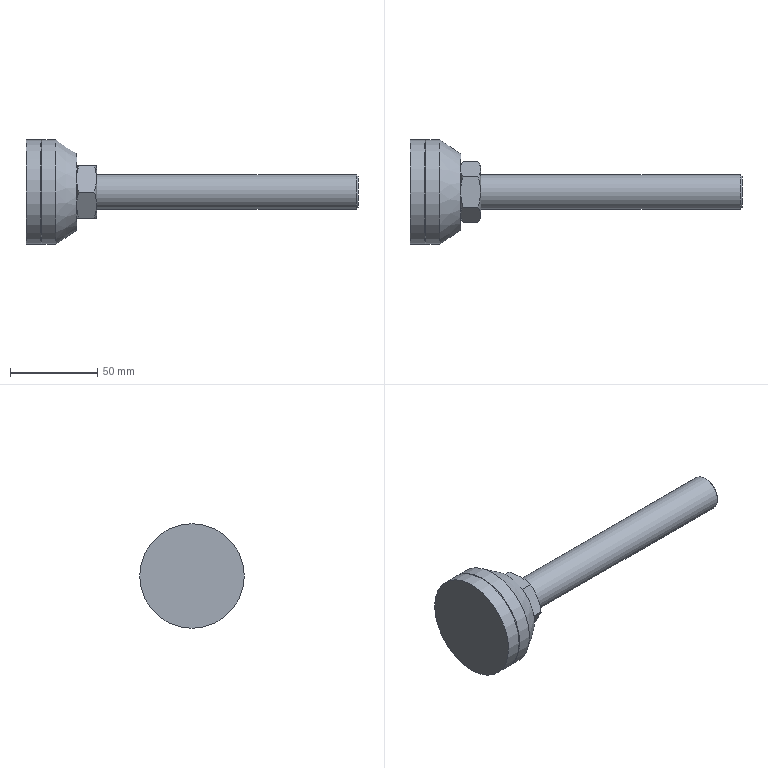Part | STEP file | C-CFJFNV60-20-150_b | 1 solid | 19 faces | box 190.5 x 60 x 60 mm | volume 129714 mm3 | plane 11 | cylinder 3 | cone 3 | torus 2 | commonest cylinder face diameters 60 x2 20 x1
STEP:
#1=CARTESIAN_POINT('',(0.,0.,-30.));
#2=VERTEX_POINT('',#1);
#3=CARTESIAN_POINT('',(0.,0.,30.));
#4=VERTEX_POINT('',#3);
#5=CARTESIAN_POINT('',(0.,0.,0.));
#6=DIRECTION('',(1.,0.,0.));
#7=DIRECTION('',(0.,0.,-1.));
#8=AXIS2_PLACEMENT_3D('',#5,#6,#7);
#9=CIRCLE('',#8,30.);
#10=EDGE_CURVE('',#2,#4,#9,.T.);
#11=ORIENTED_EDGE('',*,*,#10,.F.);
#12=CARTESIAN_POINT('',(0.,0.,0.));
#13=DIRECTION('',(1.,0.,0.));
#14=DIRECTION('',(0.,0.,-1.));
#15=AXIS2_PLACEMENT_3D('',#12,#13,#14);
#16=CIRCLE('',#15,30.);
#17=EDGE_CURVE('',#4,#2,#16,.T.);
#18=ORIENTED_EDGE('',*,*,#17,.F.);
#19=EDGE_LOOP('',(#11,#18));
#20=FACE_OUTER_BOUND('',#19,.T.);
#21=CARTESIAN_POINT('',(0.,0.,0.));
#22=DIRECTION('',(1.,0.,0.));
#23=DIRECTION('',(0.,0.,-1.));
#24=AXIS2_PLACEMENT_3D('',#21,#22,#23);
#25=PLANE('',#24);
#26=ADVANCED_FACE('',(#20),#25,.F.);
#27=CARTESIAN_POINT('',(8.5,0.,-30.));
#28=VERTEX_POINT('',#27);
#29=CARTESIAN_POINT('',(8.5,0.,30.));
#30=VERTEX_POINT('',#29);
#31=CARTESIAN_POINT('',(8.5,0.,0.));
#32=DIRECTION('',(1.,0.,0.));
#33=DIRECTION('',(0.,0.,-1.));
#34=AXIS2_PLACEMENT_3D('',#31,#32,#33);
#35=CIRCLE('',#34,30.);
#36=EDGE_CURVE('',#28,#30,#35,.T.);
#37=ORIENTED_EDGE('',*,*,#36,.F.);
#38=CARTESIAN_POINT('',(8.5,0.,0.));
#39=DIRECTION('',(1.,0.,0.));
#40=DIRECTION('',(0.,0.,-1.));
#41=AXIS2_PLACEMENT_3D('',#38,#39,#40);
#42=CIRCLE('',#41,30.);
#43=EDGE_CURVE('',#30,#28,#42,.T.);
#44=ORIENTED_EDGE('',*,*,#43,.F.);
#45=CARTESIAN_POINT('',(190.5,0.,30.));
#46=DIRECTION('',(-1.,0.,0.));
#47=VECTOR('',#46,30.);
#48=LINE('',#45,#47);
#49=EDGE_CURVE('',#30,#4,#48,.T.);
#50=ORIENTED_EDGE('',*,*,#49,.T.);
#51=ORIENTED_EDGE('',*,*,#17,.T.);
#52=ORIENTED_EDGE('',*,*,#10,.T.);
#53=ORIENTED_EDGE('',*,*,#49,.F.);
#54=EDGE_LOOP('',(#37,#44,#50,#51,#52,#53));
#55=FACE_OUTER_BOUND('',#54,.T.);
#56=CARTESIAN_POINT('',(190.5,0.,0.));
#57=DIRECTION('',(1.,0.,0.));
#58=DIRECTION('',(0.,0.,-1.));
#59=AXIS2_PLACEMENT_3D('',#56,#57,#58);
#60=CYLINDRICAL_SURFACE('',#59,30.);
#61=ADVANCED_FACE('',(#55),#60,.T.);
#62=ORIENTED_EDGE('',*,*,#36,.T.);
#63=ORIENTED_EDGE('',*,*,#43,.T.);
#64=EDGE_LOOP('',(#62,#63));
#65=FACE_OUTER_BOUND('',#64,.T.);
#66=CARTESIAN_POINT('',(8.5,0.,-29.5));
#67=VERTEX_POINT('',#66);
#68=CARTESIAN_POINT('',(8.5,0.,29.5));
#69=VERTEX_POINT('',#68);
#70=CARTESIAN_POINT('',(8.5,0.,0.));
#71=DIRECTION('',(1.,0.,0.));
#72=DIRECTION('',(0.,0.,-1.));
#73=AXIS2_PLACEMENT_3D('',#70,#71,#72);
#74=CIRCLE('',#73,29.5);
#75=EDGE_CURVE('',#67,#69,#74,.T.);
#76=ORIENTED_EDGE('',*,*,#75,.F.);
#77=CARTESIAN_POINT('',(8.5,0.,0.));
#78=DIRECTION('',(1.,0.,0.));
#79=DIRECTION('',(0.,0.,-1.));
#80=AXIS2_PLACEMENT_3D('',#77,#78,#79);
#81=CIRCLE('',#80,29.5);
#82=EDGE_CURVE('',#69,#67,#81,.T.);
#83=ORIENTED_EDGE('',*,*,#82,.F.);
#84=EDGE_LOOP('',(#76,#83));
#85=FACE_BOUND('',#84,.T.);
#86=CARTESIAN_POINT('',(8.5,30.,0.));
#87=DIRECTION('',(-1.,0.,0.));
#88=DIRECTION('',(0.,0.,1.));
#89=AXIS2_PLACEMENT_3D('',#86,#87,#88);
#90=PLANE('',#89);
#91=ADVANCED_FACE('',(#65,#85),#90,.F.);
#92=CARTESIAN_POINT('',(9.,0.,-30.));
#93=VERTEX_POINT('',#92);
#94=CARTESIAN_POINT('',(9.,0.,30.));
#95=VERTEX_POINT('',#94);
#96=CARTESIAN_POINT('',(9.,0.,0.));
#97=DIRECTION('',(1.,0.,0.));
#98=DIRECTION('',(0.,0.,-1.));
#99=AXIS2_PLACEMENT_3D('',#96,#97,#98);
#100=CIRCLE('',#99,30.);
#101=EDGE_CURVE('',#93,#95,#100,.T.);
#102=ORIENTED_EDGE('',*,*,#101,.F.);
#103=CARTESIAN_POINT('',(9.,0.,0.));
#104=DIRECTION('',(1.,0.,0.));
#105=DIRECTION('',(0.,0.,-1.));
#106=AXIS2_PLACEMENT_3D('',#103,#104,#105);
#107=CIRCLE('',#106,30.);
#108=EDGE_CURVE('',#95,#93,#107,.T.);
#109=ORIENTED_EDGE('',*,*,#108,.F.);
#110=CARTESIAN_POINT('',(8.5,0.,29.5));
#111=DIRECTION('',(-0.7071,0.,-0.7071));
#112=VECTOR('',#111,29.5);
#113=LINE('',#110,#112);
#114=EDGE_CURVE('',#95,#69,#113,.T.);
#115=ORIENTED_EDGE('',*,*,#114,.T.);
#116=ORIENTED_EDGE('',*,*,#82,.T.);
#117=ORIENTED_EDGE('',*,*,#75,.T.);
#118=ORIENTED_EDGE('',*,*,#114,.F.);
#119=EDGE_LOOP('',(#102,#109,#115,#116,#117,#118));
#120=FACE_OUTER_BOUND('',#119,.T.);
#121=CARTESIAN_POINT('',(8.5,0.,0.));
#122=DIRECTION('',(1.,0.,0.));
#123=DIRECTION('',(0.,0.,-1.));
#124=AXIS2_PLACEMENT_3D('',#121,#122,#123);
#125=CONICAL_SURFACE('',#124,29.5,0.7854);
#126=ADVANCED_FACE('',(#120),#125,.T.);
#127=CARTESIAN_POINT('',(17.,0.,-30.));
#128=VERTEX_POINT('',#127);
#129=CARTESIAN_POINT('',(17.,0.,30.));
#130=VERTEX_POINT('',#129);
#131=CARTESIAN_POINT('',(17.,0.,0.));
#132=DIRECTION('',(1.,0.,0.));
#133=DIRECTION('',(0.,0.,-1.));
#134=AXIS2_PLACEMENT_3D('',#131,#132,#133);
#135=CIRCLE('',#134,30.);
#136=EDGE_CURVE('',#128,#130,#135,.T.);
#137=ORIENTED_EDGE('',*,*,#136,.F.);
#138=CARTESIAN_POINT('',(17.,0.,0.));
#139=DIRECTION('',(1.,0.,0.));
#140=DIRECTION('',(0.,0.,-1.));
#141=AXIS2_PLACEMENT_3D('',#138,#139,#140);
#142=CIRCLE('',#141,30.);
#143=EDGE_CURVE('',#130,#128,#142,.T.);
#144=ORIENTED_EDGE('',*,*,#143,.F.);
#145=CARTESIAN_POINT('',(190.5,0.,30.));
#146=DIRECTION('',(-1.,0.,0.));
#147=VECTOR('',#146,30.);
#148=LINE('',#145,#147);
#149=EDGE_CURVE('',#130,#95,#148,.T.);
#150=ORIENTED_EDGE('',*,*,#149,.T.);
#151=ORIENTED_EDGE('',*,*,#108,.T.);
#152=ORIENTED_EDGE('',*,*,#101,.T.);
#153=ORIENTED_EDGE('',*,*,#149,.F.);
#154=EDGE_LOOP('',(#137,#144,#150,#151,#152,#153));
#155=FACE_OUTER_BOUND('',#154,.T.);
#156=CARTESIAN_POINT('',(190.5,0.,0.));
#157=DIRECTION('',(1.,0.,0.));
#158=DIRECTION('',(0.,0.,-1.));
#159=AXIS2_PLACEMENT_3D('',#156,#157,#158);
#160=CYLINDRICAL_SURFACE('',#159,30.);
#161=ADVANCED_FACE('',(#155),#160,.T.);
#162=ORIENTED_EDGE('',*,*,#136,.T.);
#163=ORIENTED_EDGE('',*,*,#143,.T.);
#164=CARTESIAN_POINT('',(29.,0.,-22.));
#165=VERTEX_POINT('',#164);
#166=CARTESIAN_POINT('',(17.,0.,-30.));
#167=DIRECTION('',(0.8321,0.,0.5547));
#168=VECTOR('',#167,30.);
#169=LINE('',#166,#168);
#170=EDGE_CURVE('',#128,#165,#169,.T.);
#171=ORIENTED_EDGE('',*,*,#170,.T.);
#172=CARTESIAN_POINT('',(29.,0.,0.));
#173=DIRECTION('',(1.,0.,0.));
#174=DIRECTION('',(0.,0.,-1.));
#175=AXIS2_PLACEMENT_3D('',#172,#173,#174);
#176=CIRCLE('',#175,22.);
#177=EDGE_CURVE('',#165,#165,#176,.T.);
#178=ORIENTED_EDGE('',*,*,#177,.F.);
#179=ORIENTED_EDGE('',*,*,#170,.F.);
#180=EDGE_LOOP('',(#162,#163,#171,#178,#179));
#181=FACE_OUTER_BOUND('',#180,.T.);
#182=CARTESIAN_POINT('',(17.,0.,0.));
#183=DIRECTION('',(-1.,0.,0.));
#184=DIRECTION('',(0.,0.,1.));
#185=AXIS2_PLACEMENT_3D('',#182,#183,#184);
#186=CONICAL_SURFACE('',#185,30.,0.588);
#187=ADVANCED_FACE('',(#181),#186,.T.);
#188=ORIENTED_EDGE('',*,*,#177,.T.);
#189=EDGE_LOOP('',(#188));
#190=FACE_OUTER_BOUND('',#189,.T.);
#191=CARTESIAN_POINT('',(29.,0.,-13.821));
#192=VERTEX_POINT('',#191);
#193=CARTESIAN_POINT('',(29.,0.,13.821));
#194=VERTEX_POINT('',#193);
#195=CARTESIAN_POINT('',(29.,0.,0.));
#196=DIRECTION('',(1.,0.,0.));
#197=DIRECTION('',(0.,0.,-1.));
#198=AXIS2_PLACEMENT_3D('',#195,#196,#197);
#199=CIRCLE('',#198,13.821);
#200=EDGE_CURVE('',#192,#194,#199,.T.);
#201=ORIENTED_EDGE('',*,*,#200,.F.);
#202=CARTESIAN_POINT('',(29.,0.,0.));
#203=DIRECTION('',(1.,0.,0.));
#204=DIRECTION('',(0.,0.,-1.));
#205=AXIS2_PLACEMENT_3D('',#202,#203,#204);
#206=CIRCLE('',#205,13.821);
#207=EDGE_CURVE('',#194,#192,#206,.T.);
#208=ORIENTED_EDGE('',*,*,#207,.F.);
#209=EDGE_LOOP('',(#201,#208));
#210=FACE_BOUND('',#209,.T.);
#211=CARTESIAN_POINT('',(29.,22.,0.));
#212=DIRECTION('',(-1.,0.,0.));
#213=DIRECTION('',(0.,0.,1.));
#214=AXIS2_PLACEMENT_3D('',#211,#212,#213);
#215=PLANE('',#214);
#216=ADVANCED_FACE('',(#190,#210),#215,.F.);
#217=CARTESIAN_POINT('',(30.5,8.66,15.));
#218=VERTEX_POINT('',#217);
#219=CARTESIAN_POINT('',(29.146,0.,15.));
#220=VERTEX_POINT('',#219);
#221=CARTESIAN_POINT('',(30.5,8.66,15.));
#222=CARTESIAN_POINT('',(30.391,8.453,15.));
#223=CARTESIAN_POINT('',(30.295,8.244,15.));
#224=CARTESIAN_POINT('',(29.715,6.855,15.));
#225=CARTESIAN_POINT('',(29.46,5.487,15.));
#226=CARTESIAN_POINT('',(29.179,2.703,15.));
#227=CARTESIAN_POINT('',(29.146,1.288,15.));
#228=CARTESIAN_POINT('',(29.146,0.,15.));
#229=B_SPLINE_CURVE_WITH_KNOTS('',3,(#221,#222,#223,#224,#225,#226,#227,#228),.UNSPECIFIED.,.F.,.F.,(4,2,2,4),(4.146,4.211,4.598,4.984),.UNSPECIFIED.);
#230=EDGE_CURVE('',#218,#220,#229,.T.);
#231=ORIENTED_EDGE('',*,*,#230,.F.);
#232=CARTESIAN_POINT('',(30.5,17.321,0.));
#233=VERTEX_POINT('',#232);
#234=CARTESIAN_POINT('',(30.5,17.321,0.));
#235=CARTESIAN_POINT('',(30.391,17.217,0.1798));
#236=CARTESIAN_POINT('',(30.295,17.112,0.3609));
#237=CARTESIAN_POINT('',(29.715,16.418,1.564));
#238=CARTESIAN_POINT('',(29.46,15.734,2.748));
#239=CARTESIAN_POINT('',(29.179,14.342,5.159));
#240=CARTESIAN_POINT('',(29.146,13.634,6.385));
#241=CARTESIAN_POINT('',(29.146,12.99,7.5));
#242=CARTESIAN_POINT('',(29.146,12.346,8.615));
#243=CARTESIAN_POINT('',(29.179,11.639,9.841));
#244=CARTESIAN_POINT('',(29.46,10.247,12.252));
#245=CARTESIAN_POINT('',(29.715,9.563,13.436));
#246=CARTESIAN_POINT('',(30.295,8.869,14.639));
#247=CARTESIAN_POINT('',(30.391,8.764,14.82));
#248=CARTESIAN_POINT('',(30.5,8.66,15.));
#249=B_SPLINE_CURVE_WITH_KNOTS('',3,(#234,#235,#236,#237,#238,#239,#240,#241,#242,#243,#244,#245,#246,#247,#248),.UNSPECIFIED.,.F.,.F.,(4,2,2,3,2,2,4),(4.146,4.211,4.598,4.984,5.37,5.757,5.822),.UNSPECIFIED.);
#250=EDGE_CURVE('',#233,#218,#249,.T.);
#251=ORIENTED_EDGE('',*,*,#250,.F.);
#252=CARTESIAN_POINT('',(30.5,8.66,-15.));
#253=VERTEX_POINT('',#252);
#254=CARTESIAN_POINT('',(30.5,8.66,-15.));
#255=CARTESIAN_POINT('',(30.391,8.764,-14.82));
#256=CARTESIAN_POINT('',(30.295,8.869,-14.639));
#257=CARTESIAN_POINT('',(29.715,9.563,-13.436));
#258=CARTESIAN_POINT('',(29.46,10.247,-12.252));
#259=CARTESIAN_POINT('',(29.179,11.639,-9.841));
#260=CARTESIAN_POINT('',(29.146,12.346,-8.615));
#261=CARTESIAN_POINT('',(29.146,12.99,-7.5));
#262=CARTESIAN_POINT('',(29.146,13.634,-6.385));
#263=CARTESIAN_POINT('',(29.179,14.342,-5.159));
#264=CARTESIAN_POINT('',(29.46,15.734,-2.748));
#265=CARTESIAN_POINT('',(29.715,16.418,-1.564));
#266=CARTESIAN_POINT('',(30.295,17.112,-0.3609));
#267=CARTESIAN_POINT('',(30.391,17.217,-0.1798));
#268=CARTESIAN_POINT('',(30.5,17.321,0.));
#269=B_SPLINE_CURVE_WITH_KNOTS('',3,(#254,#255,#256,#257,#258,#259,#260,#261,#262,#263,#264,#265,#266,#267,#268),.UNSPECIFIED.,.F.,.F.,(4,2,2,3,2,2,4),(4.146,4.211,4.598,4.984,5.37,5.757,5.822),.UNSPECIFIED.);
#270=EDGE_CURVE('',#253,#233,#269,.T.);
#271=ORIENTED_EDGE('',*,*,#270,.F.);
#272=CARTESIAN_POINT('',(30.5,-8.66,-15.));
#273=VERTEX_POINT('',#272);
#274=CARTESIAN_POINT('',(30.5,-8.66,-15.));
#275=CARTESIAN_POINT('',(30.391,-8.453,-15.));
#276=CARTESIAN_POINT('',(30.295,-8.244,-15.));
#277=CARTESIAN_POINT('',(29.715,-6.855,-15.));
#278=CARTESIAN_POINT('',(29.46,-5.487,-15.));
#279=CARTESIAN_POINT('',(29.179,-2.703,-15.));
#280=CARTESIAN_POINT('',(29.146,-1.288,-15.));
#281=CARTESIAN_POINT('',(29.146,0.,-15.));
#282=CARTESIAN_POINT('',(29.146,1.288,-15.));
#283=CARTESIAN_POINT('',(29.179,2.703,-15.));
#284=CARTESIAN_POINT('',(29.46,5.487,-15.));
#285=CARTESIAN_POINT('',(29.715,6.855,-15.));
#286=CARTESIAN_POINT('',(30.295,8.244,-15.));
#287=CARTESIAN_POINT('',(30.391,8.453,-15.));
#288=CARTESIAN_POINT('',(30.5,8.66,-15.));
#289=B_SPLINE_CURVE_WITH_KNOTS('',3,(#274,#275,#276,#277,#278,#279,#280,#281,#282,#283,#284,#285,#286,#287,#288),.UNSPECIFIED.,.F.,.F.,(4,2,2,3,2,2,4),(4.146,4.211,4.598,4.984,5.37,5.757,5.822),.UNSPECIFIED.);
#290=EDGE_CURVE('',#273,#253,#289,.T.);
#291=ORIENTED_EDGE('',*,*,#290,.F.);
#292=CARTESIAN_POINT('',(30.5,-17.321,0.));
#293=VERTEX_POINT('',#292);
#294=CARTESIAN_POINT('',(30.5,-17.321,0.));
#295=CARTESIAN_POINT('',(30.391,-17.217,-0.1798));
#296=CARTESIAN_POINT('',(30.295,-17.112,-0.3609));
#297=CARTESIAN_POINT('',(29.715,-16.418,-1.564));
#298=CARTESIAN_POINT('',(29.46,-15.734,-2.748));
#299=CARTESIAN_POINT('',(29.179,-14.342,-5.159));
#300=CARTESIAN_POINT('',(29.146,-13.634,-6.385));
#301=CARTESIAN_POINT('',(29.146,-12.99,-7.5));
#302=CARTESIAN_POINT('',(29.146,-12.346,-8.615));
#303=CARTESIAN_POINT('',(29.179,-11.639,-9.841));
#304=CARTESIAN_POINT('',(29.46,-10.247,-12.252));
#305=CARTESIAN_POINT('',(29.715,-9.563,-13.436));
#306=CARTESIAN_POINT('',(30.295,-8.869,-14.639));
#307=CARTESIAN_POINT('',(30.391,-8.764,-14.82));
#308=CARTESIAN_POINT('',(30.5,-8.66,-15.));
#309=B_SPLINE_CURVE_WITH_KNOTS('',3,(#294,#295,#296,#297,#298,#299,#300,#301,#302,#303,#304,#305,#306,#307,#308),.UNSPECIFIED.,.F.,.F.,(4,2,2,3,2,2,4),(4.146,4.211,4.598,4.984,5.37,5.757,5.822),.UNSPECIFIED.);
#310=EDGE_CURVE('',#293,#273,#309,.T.);
#311=ORIENTED_EDGE('',*,*,#310,.F.);
#312=CARTESIAN_POINT('',(30.5,-8.66,15.));
#313=VERTEX_POINT('',#312);
#314=CARTESIAN_POINT('',(30.5,-8.66,15.));
#315=CARTESIAN_POINT('',(30.391,-8.764,14.82));
#316=CARTESIAN_POINT('',(30.295,-8.869,14.639));
#317=CARTESIAN_POINT('',(29.715,-9.563,13.436));
#318=CARTESIAN_POINT('',(29.46,-10.247,12.252));
#319=CARTESIAN_POINT('',(29.179,-11.639,9.841));
#320=CARTESIAN_POINT('',(29.146,-12.346,8.615));
#321=CARTESIAN_POINT('',(29.146,-12.99,7.5));
#322=CARTESIAN_POINT('',(29.146,-13.634,6.385));
#323=CARTESIAN_POINT('',(29.179,-14.342,5.159));
#324=CARTESIAN_POINT('',(29.46,-15.734,2.748));
#325=CARTESIAN_POINT('',(29.715,-16.418,1.564));
#326=CARTESIAN_POINT('',(30.295,-17.112,0.3609));
#327=CARTESIAN_POINT('',(30.391,-17.217,0.1798));
#328=CARTESIAN_POINT('',(30.5,-17.321,0.));
#329=B_SPLINE_CURVE_WITH_KNOTS('',3,(#314,#315,#316,#317,#318,#319,#320,#321,#322,#323,#324,#325,#326,#327,#328),.UNSPECIFIED.,.F.,.F.,(4,2,2,3,2,2,4),(4.146,4.211,4.598,4.984,5.37,5.757,5.822),.UNSPECIFIED.);
#330=EDGE_CURVE('',#313,#293,#329,.T.);
#331=ORIENTED_EDGE('',*,*,#330,.F.);
#332=CARTESIAN_POINT('',(29.146,0.,15.));
#333=CARTESIAN_POINT('',(29.146,-1.288,15.));
#334=CARTESIAN_POINT('',(29.179,-2.703,15.));
#335=CARTESIAN_POINT('',(29.46,-5.487,15.));
#336=CARTESIAN_POINT('',(29.715,-6.855,15.));
#337=CARTESIAN_POINT('',(30.295,-8.244,15.));
#338=CARTESIAN_POINT('',(30.391,-8.453,15.));
#339=CARTESIAN_POINT('',(30.5,-8.66,15.));
#340=B_SPLINE_CURVE_WITH_KNOTS('',3,(#332,#333,#334,#335,#336,#337,#338,#339),.UNSPECIFIED.,.F.,.F.,(4,2,2,4),(4.984,5.37,5.757,5.822),.UNSPECIFIED.);
#341=EDGE_CURVE('',#220,#313,#340,.T.);
#342=ORIENTED_EDGE('',*,*,#341,.F.);
#343=CARTESIAN_POINT('',(33.833,0.,13.821));
#344=DIRECTION('',(0.,-1.,0.));
#345=DIRECTION('',(0.,0.,1.));
#346=AXIS2_PLACEMENT_3D('',#343,#344,#345);
#347=CIRCLE('',#346,4.833);
#348=EDGE_CURVE('',#220,#194,#347,.T.);
#349=ORIENTED_EDGE('',*,*,#348,.T.);
#350=ORIENTED_EDGE('',*,*,#207,.T.);
#351=ORIENTED_EDGE('',*,*,#200,.T.);
#352=ORIENTED_EDGE('',*,*,#348,.F.);
#353=EDGE_LOOP('',(#231,#251,#271,#291,#311,#331,#342,#349,#350,#351,#352));
#354=FACE_OUTER_BOUND('',#353,.T.);
#355=CARTESIAN_POINT('',(33.833,0.,0.));
#356=DIRECTION('',(1.,0.,0.));
#357=DIRECTION('',(0.,0.,-1.));
#358=AXIS2_PLACEMENT_3D('',#355,#356,#357);
#359=TOROIDAL_SURFACE('',#358,13.821,4.833);
#360=ADVANCED_FACE('',(#354),#359,.T.);
#361=ORIENTED_EDGE('',*,*,#230,.T.);
#362=ORIENTED_EDGE('',*,*,#341,.T.);
#363=CARTESIAN_POINT('',(39.,-8.66,15.));
#364=VERTEX_POINT('',#363);
#365=CARTESIAN_POINT('',(40.5,-8.66,15.));
#366=DIRECTION('',(-1.,0.,0.));
#367=VECTOR('',#366,1000.);
#368=LINE('',#365,#367);
#369=EDGE_CURVE('',#364,#313,#368,.T.);
#370=ORIENTED_EDGE('',*,*,#369,.F.);
#371=CARTESIAN_POINT('',(40.354,0.,15.));
#372=VERTEX_POINT('',#371);
#373=CARTESIAN_POINT('',(39.,-8.66,15.));
#374=CARTESIAN_POINT('',(39.109,-8.453,15.));
#375=CARTESIAN_POINT('',(39.205,-8.244,15.));
#376=CARTESIAN_POINT('',(39.785,-6.855,15.));
#377=CARTESIAN_POINT('',(40.04,-5.487,15.));
#378=CARTESIAN_POINT('',(40.321,-2.703,15.));
#379=CARTESIAN_POINT('',(40.354,-1.288,15.));
#380=CARTESIAN_POINT('',(40.354,0.,15.));
#381=B_SPLINE_CURVE_WITH_KNOTS('',3,(#373,#374,#375,#376,#377,#378,#379,#380),.UNSPECIFIED.,.F.,.F.,(4,2,2,4),(-3.33,-3.265,-2.878,-2.492),.UNSPECIFIED.);
#382=EDGE_CURVE('',#364,#372,#381,.T.);
#383=ORIENTED_EDGE('',*,*,#382,.T.);
#384=CARTESIAN_POINT('',(39.,8.66,15.));
#385=VERTEX_POINT('',#384);
#386=CARTESIAN_POINT('',(40.354,0.,15.));
#387=CARTESIAN_POINT('',(40.354,1.288,15.));
#388=CARTESIAN_POINT('',(40.321,2.703,15.));
#389=CARTESIAN_POINT('',(40.04,5.487,15.));
#390=CARTESIAN_POINT('',(39.785,6.855,15.));
#391=CARTESIAN_POINT('',(39.205,8.244,15.));
#392=CARTESIAN_POINT('',(39.109,8.453,15.));
#393=CARTESIAN_POINT('',(39.,8.66,15.));
#394=B_SPLINE_CURVE_WITH_KNOTS('',3,(#386,#387,#388,#389,#390,#391,#392,#393),.UNSPECIFIED.,.F.,.F.,(4,2,2,4),(-2.492,-2.106,-1.719,-1.654),.UNSPECIFIED.);
#395=EDGE_CURVE('',#372,#385,#394,.T.);
#396=ORIENTED_EDGE('',*,*,#395,.T.);
#397=CARTESIAN_POINT('',(40.5,8.66,15.));
#398=DIRECTION('',(-1.,0.,0.));
#399=VECTOR('',#398,1000.);
#400=LINE('',#397,#399);
#401=EDGE_CURVE('',#385,#218,#400,.T.);
#402=ORIENTED_EDGE('',*,*,#401,.T.);
#403=EDGE_LOOP('',(#361,#362,#370,#383,#396,#402));
#404=FACE_OUTER_BOUND('',#403,.T.);
#405=CARTESIAN_POINT('',(40.5,8.66,15.));
#406=DIRECTION('',(0.,0.,-1.));
#407=DIRECTION('',(-1.,0.,0.));
#408=AXIS2_PLACEMENT_3D('',#405,#406,#407);
#409=PLANE('',#408);
#410=ADVANCED_FACE('',(#404),#409,.F.);
#411=ORIENTED_EDGE('',*,*,#250,.T.);
#412=ORIENTED_EDGE('',*,*,#401,.F.);
#413=CARTESIAN_POINT('',(39.,17.321,0.));
#414=VERTEX_POINT('',#413);
#415=CARTESIAN_POINT('',(39.,8.66,15.));
#416=CARTESIAN_POINT('',(39.109,8.764,14.82));
#417=CARTESIAN_POINT('',(39.205,8.869,14.639));
#418=CARTESIAN_POINT('',(39.785,9.563,13.436));
#419=CARTESIAN_POINT('',(40.04,10.247,12.252));
#420=CARTESIAN_POINT('',(40.321,11.639,9.841));
#421=CARTESIAN_POINT('',(40.354,12.346,8.615));
#422=CARTESIAN_POINT('',(40.354,13.634,6.385));
#423=CARTESIAN_POINT('',(40.321,14.342,5.159));
#424=CARTESIAN_POINT('',(40.04,15.734,2.748));
#425=CARTESIAN_POINT('',(39.785,16.418,1.564));
#426=CARTESIAN_POINT('',(39.205,17.112,0.3609));
#427=CARTESIAN_POINT('',(39.109,17.217,0.1798));
#428=CARTESIAN_POINT('',(39.,17.321,0.));
#429=B_SPLINE_CURVE_WITH_KNOTS('',3,(#415,#416,#417,#418,#419,#420,#421,#422,#423,#424,#425,#426,#427,#428),.UNSPECIFIED.,.F.,.F.,(4,2,2,2,2,2,4),(-3.33,-3.265,-2.878,-2.492,-2.106,-1.719,-1.654),.UNSPECIFIED.);
#430=EDGE_CURVE('',#385,#414,#429,.T.);
#431=ORIENTED_EDGE('',*,*,#430,.T.);
#432=CARTESIAN_POINT('',(40.5,17.321,0.));
#433=DIRECTION('',(-1.,0.,0.));
#434=VECTOR('',#433,1000.);
#435=LINE('',#432,#434);
#436=EDGE_CURVE('',#414,#233,#435,.T.);
#437=ORIENTED_EDGE('',*,*,#436,.T.);
#438=EDGE_LOOP('',(#411,#412,#431,#437));
#439=FACE_OUTER_BOUND('',#438,.T.);
#440=CARTESIAN_POINT('',(40.5,17.321,0.));
#441=DIRECTION('',(0.,-0.866,-0.5));
#442=DIRECTION('',(0.,0.5,-0.866));
#443=AXIS2_PLACEMENT_3D('',#440,#441,#442);
#444=PLANE('',#443);
#445=ADVANCED_FACE('',(#439),#444,.F.);
#446=ORIENTED_EDGE('',*,*,#270,.T.);
#447=ORIENTED_EDGE('',*,*,#436,.F.);
#448=CARTESIAN_POINT('',(39.,8.66,-15.));
#449=VERTEX_POINT('',#448);
#450=CARTESIAN_POINT('',(39.,17.321,0.));
#451=CARTESIAN_POINT('',(39.109,17.217,-0.1798));
#452=CARTESIAN_POINT('',(39.205,17.112,-0.3609));
#453=CARTESIAN_POINT('',(39.785,16.418,-1.564));
#454=CARTESIAN_POINT('',(40.04,15.734,-2.748));
#455=CARTESIAN_POINT('',(40.321,14.342,-5.159));
#456=CARTESIAN_POINT('',(40.354,13.634,-6.385));
#457=CARTESIAN_POINT('',(40.354,12.346,-8.615));
#458=CARTESIAN_POINT('',(40.321,11.639,-9.841));
#459=CARTESIAN_POINT('',(40.04,10.247,-12.252));
#460=CARTESIAN_POINT('',(39.785,9.563,-13.436));
#461=CARTESIAN_POINT('',(39.205,8.869,-14.639));
#462=CARTESIAN_POINT('',(39.109,8.764,-14.82));
#463=CARTESIAN_POINT('',(39.,8.66,-15.));
#464=B_SPLINE_CURVE_WITH_KNOTS('',3,(#450,#451,#452,#453,#454,#455,#456,#457,#458,#459,#460,#461,#462,#463),.UNSPECIFIED.,.F.,.F.,(4,2,2,2,2,2,4),(-3.33,-3.265,-2.878,-2.492,-2.106,-1.719,-1.654),.UNSPECIFIED.);
#465=EDGE_CURVE('',#414,#449,#464,.T.);
#466=ORIENTED_EDGE('',*,*,#465,.T.);
#467=CARTESIAN_POINT('',(40.5,8.66,-15.));
#468=DIRECTION('',(-1.,0.,0.));
#469=VECTOR('',#468,1000.);
#470=LINE('',#467,#469);
#471=EDGE_CURVE('',#449,#253,#470,.T.);
#472=ORIENTED_EDGE('',*,*,#471,.T.);
#473=EDGE_LOOP('',(#446,#447,#466,#472));
#474=FACE_OUTER_BOUND('',#473,.T.);
#475=CARTESIAN_POINT('',(40.5,8.66,-15.));
#476=DIRECTION('',(0.,-0.866,0.5));
#477=DIRECTION('',(0.,-0.5,-0.866));
#478=AXIS2_PLACEMENT_3D('',#475,#476,#477);
#479=PLANE('',#478);
#480=ADVANCED_FACE('',(#474),#479,.F.);
#481=ORIENTED_EDGE('',*,*,#290,.T.);
#482=ORIENTED_EDGE('',*,*,#471,.F.);
#483=CARTESIAN_POINT('',(39.,-8.66,-15.));
#484=VERTEX_POINT('',#483);
#485=CARTESIAN_POINT('',(39.,8.66,-15.));
#486=CARTESIAN_POINT('',(39.109,8.453,-15.));
#487=CARTESIAN_POINT('',(39.205,8.244,-15.));
#488=CARTESIAN_POINT('',(39.785,6.855,-15.));
#489=CARTESIAN_POINT('',(40.04,5.487,-15.));
#490=CARTESIAN_POINT('',(40.321,2.703,-15.));
#491=CARTESIAN_POINT('',(40.354,1.288,-15.));
#492=CARTESIAN_POINT('',(40.354,-1.288,-15.));
#493=CARTESIAN_POINT('',(40.321,-2.703,-15.));
#494=CARTESIAN_POINT('',(40.04,-5.487,-15.));
#495=CARTESIAN_POINT('',(39.785,-6.855,-15.));
#496=CARTESIAN_POINT('',(39.205,-8.244,-15.));
#497=CARTESIAN_POINT('',(39.109,-8.453,-15.));
#498=CARTESIAN_POINT('',(39.,-8.66,-15.));
#499=B_SPLINE_CURVE_WITH_KNOTS('',3,(#485,#486,#487,#488,#489,#490,#491,#492,#493,#494,#495,#496,#497,#498),.UNSPECIFIED.,.F.,.F.,(4,2,2,2,2,2,4),(-3.33,-3.265,-2.878,-2.492,-2.106,-1.719,-1.654),.UNSPECIFIED.);
#500=EDGE_CURVE('',#449,#484,#499,.T.);
#501=ORIENTED_EDGE('',*,*,#500,.T.);
#502=CARTESIAN_POINT('',(40.5,-8.66,-15.));
#503=DIRECTION('',(-1.,0.,0.));
#504=VECTOR('',#503,1000.);
#505=LINE('',#502,#504);
#506=EDGE_CURVE('',#484,#273,#505,.T.);
#507=ORIENTED_EDGE('',*,*,#506,.T.);
#508=EDGE_LOOP('',(#481,#482,#501,#507));
#509=FACE_OUTER_BOUND('',#508,.T.);
#510=CARTESIAN_POINT('',(40.5,-8.66,-15.));
#511=DIRECTION('',(0.,0.,1.));
#512=DIRECTION('',(1.,0.,0.));
#513=AXIS2_PLACEMENT_3D('',#510,#511,#512);
#514=PLANE('',#513);
#515=ADVANCED_FACE('',(#509),#514,.F.);
#516=ORIENTED_EDGE('',*,*,#310,.T.);
#517=ORIENTED_EDGE('',*,*,#506,.F.);
#518=CARTESIAN_POINT('',(39.,-17.321,0.));
#519=VERTEX_POINT('',#518);
#520=CARTESIAN_POINT('',(39.,-8.66,-15.));
#521=CARTESIAN_POINT('',(39.109,-8.764,-14.82));
#522=CARTESIAN_POINT('',(39.205,-8.869,-14.639));
#523=CARTESIAN_POINT('',(39.785,-9.563,-13.436));
#524=CARTESIAN_POINT('',(40.04,-10.247,-12.252));
#525=CARTESIAN_POINT('',(40.321,-11.639,-9.841));
#526=CARTESIAN_POINT('',(40.354,-12.346,-8.615));
#527=CARTESIAN_POINT('',(40.354,-13.634,-6.385));
#528=CARTESIAN_POINT('',(40.321,-14.342,-5.159));
#529=CARTESIAN_POINT('',(40.04,-15.734,-2.748));
#530=CARTESIAN_POINT('',(39.785,-16.418,-1.564));
#531=CARTESIAN_POINT('',(39.205,-17.112,-0.3609));
#532=CARTESIAN_POINT('',(39.109,-17.217,-0.1798));
#533=CARTESIAN_POINT('',(39.,-17.321,0.));
#534=B_SPLINE_CURVE_WITH_KNOTS('',3,(#520,#521,#522,#523,#524,#525,#526,#527,#528,#529,#530,#531,#532,#533),.UNSPECIFIED.,.F.,.F.,(4,2,2,2,2,2,4),(-3.33,-3.265,-2.878,-2.492,-2.106,-1.719,-1.654),.UNSPECIFIED.);
#535=EDGE_CURVE('',#484,#519,#534,.T.);
#536=ORIENTED_EDGE('',*,*,#535,.T.);
#537=CARTESIAN_POINT('',(40.5,-17.321,0.));
#538=DIRECTION('',(-1.,0.,0.));
#539=VECTOR('',#538,1000.);
#540=LINE('',#537,#539);
#541=EDGE_CURVE('',#519,#293,#540,.T.);
#542=ORIENTED_EDGE('',*,*,#541,.T.);
#543=EDGE_LOOP('',(#516,#517,#536,#542));
#544=FACE_OUTER_BOUND('',#543,.T.);
#545=CARTESIAN_POINT('',(40.5,-17.321,0.));
#546=DIRECTION('',(0.,0.866,0.5));
#547=DIRECTION('',(0.,-0.5,0.866));
#548=AXIS2_PLACEMENT_3D('',#545,#546,#547);
#549=PLANE('',#548);
#550=ADVANCED_FACE('',(#544),#549,.F.);
#551=ORIENTED_EDGE('',*,*,#330,.T.);
#552=ORIENTED_EDGE('',*,*,#541,.F.);
#553=CARTESIAN_POINT('',(39.,-17.321,0.));
#554=CARTESIAN_POINT('',(39.109,-17.217,0.1798));
#555=CARTESIAN_POINT('',(39.205,-17.112,0.3609));
#556=CARTESIAN_POINT('',(39.785,-16.418,1.564));
#557=CARTESIAN_POINT('',(40.04,-15.734,2.748));
#558=CARTESIAN_POINT('',(40.321,-14.342,5.159));
#559=CARTESIAN_POINT('',(40.354,-13.634,6.385));
#560=CARTESIAN_POINT('',(40.354,-12.346,8.615));
#561=CARTESIAN_POINT('',(40.321,-11.639,9.841));
#562=CARTESIAN_POINT('',(40.04,-10.247,12.252));
#563=CARTESIAN_POINT('',(39.785,-9.563,13.436));
#564=CARTESIAN_POINT('',(39.205,-8.869,14.639));
#565=CARTESIAN_POINT('',(39.109,-8.764,14.82));
#566=CARTESIAN_POINT('',(39.,-8.66,15.));
#567=B_SPLINE_CURVE_WITH_KNOTS('',3,(#553,#554,#555,#556,#557,#558,#559,#560,#561,#562,#563,#564,#565,#566),.UNSPECIFIED.,.F.,.F.,(4,2,2,2,2,2,4),(-3.33,-3.265,-2.878,-2.492,-2.106,-1.719,-1.654),.UNSPECIFIED.);
#568=EDGE_CURVE('',#519,#364,#567,.T.);
#569=ORIENTED_EDGE('',*,*,#568,.T.);
#570=ORIENTED_EDGE('',*,*,#369,.T.);
#571=EDGE_LOOP('',(#551,#552,#569,#570));
#572=FACE_OUTER_BOUND('',#571,.T.);
#573=CARTESIAN_POINT('',(40.5,-8.66,15.));
#574=DIRECTION('',(0.,0.866,-0.5));
#575=DIRECTION('',(0.,0.5,0.866));
#576=AXIS2_PLACEMENT_3D('',#573,#574,#575);
#577=PLANE('',#576);
#578=ADVANCED_FACE('',(#572),#577,.F.);
#579=CARTESIAN_POINT('',(190.5,0.,-9.));
#580=VERTEX_POINT('',#579);
#581=CARTESIAN_POINT('',(190.5,0.,0.));
#582=DIRECTION('',(1.,0.,0.));
#583=DIRECTION('',(0.,0.,-1.));
#584=AXIS2_PLACEMENT_3D('',#581,#582,#583);
#585=CIRCLE('',#584,9.);
#586=EDGE_CURVE('',#580,#580,#585,.T.);
#587=ORIENTED_EDGE('',*,*,#586,.T.);
#588=EDGE_LOOP('',(#587));
#589=FACE_OUTER_BOUND('',#588,.T.);
#590=CARTESIAN_POINT('',(190.5,9.,0.));
#591=DIRECTION('',(-1.,0.,0.));
#592=DIRECTION('',(0.,0.,1.));
#593=AXIS2_PLACEMENT_3D('',#590,#591,#592);
#594=PLANE('',#593);
#595=ADVANCED_FACE('',(#589),#594,.F.);
#596=CARTESIAN_POINT('',(189.5,0.,-10.));
#597=VERTEX_POINT('',#596);
#598=CARTESIAN_POINT('',(189.5,0.,10.));
#599=VERTEX_POINT('',#598);
#600=CARTESIAN_POINT('',(189.5,0.,0.));
#601=DIRECTION('',(1.,0.,0.));
#602=DIRECTION('',(0.,0.,-1.));
#603=AXIS2_PLACEMENT_3D('',#600,#601,#602);
#604=CIRCLE('',#603,10.);
#605=EDGE_CURVE('',#597,#599,#604,.T.);
#606=ORIENTED_EDGE('',*,*,#605,.T.);
#607=CARTESIAN_POINT('',(189.5,0.,0.));
#608=DIRECTION('',(1.,0.,0.));
#609=DIRECTION('',(0.,0.,-1.));
#610=AXIS2_PLACEMENT_3D('',#607,#608,#609);
#611=CIRCLE('',#610,10.);
#612=EDGE_CURVE('',#599,#597,#611,.T.);
#613=ORIENTED_EDGE('',*,*,#612,.T.);
#614=CARTESIAN_POINT('',(189.5,0.,-10.));
#615=DIRECTION('',(0.7071,0.,0.7071));
#616=VECTOR('',#615,10.);
#617=LINE('',#614,#616);
#618=EDGE_CURVE('',#597,#580,#617,.T.);
#619=ORIENTED_EDGE('',*,*,#618,.T.);
#620=ORIENTED_EDGE('',*,*,#586,.F.);
#621=ORIENTED_EDGE('',*,*,#618,.F.);
#622=EDGE_LOOP('',(#606,#613,#619,#620,#621));
#623=FACE_OUTER_BOUND('',#622,.T.);
#624=CARTESIAN_POINT('',(189.5,0.,0.));
#625=DIRECTION('',(-1.,0.,0.));
#626=DIRECTION('',(0.,0.,1.));
#627=AXIS2_PLACEMENT_3D('',#624,#625,#626);
#628=CONICAL_SURFACE('',#627,10.,0.7854);
#629=ADVANCED_FACE('',(#623),#628,.T.);
#630=ORIENTED_EDGE('',*,*,#605,.F.);
#631=ORIENTED_EDGE('',*,*,#612,.F.);
#632=CARTESIAN_POINT('',(40.5,0.,10.));
#633=VERTEX_POINT('',#632);
#634=CARTESIAN_POINT('',(190.5,0.,10.));
#635=DIRECTION('',(-1.,0.,0.));
#636=VECTOR('',#635,10.);
#637=LINE('',#634,#636);
#638=EDGE_CURVE('',#599,#633,#637,.T.);
#639=ORIENTED_EDGE('',*,*,#638,.T.);
#640=CARTESIAN_POINT('',(40.5,0.,-10.));
#641=VERTEX_POINT('',#640);
#642=CARTESIAN_POINT('',(40.5,0.,0.));
#643=DIRECTION('',(1.,0.,0.));
#644=DIRECTION('',(0.,0.,-1.));
#645=AXIS2_PLACEMENT_3D('',#642,#643,#644);
#646=CIRCLE('',#645,10.);
#647=EDGE_CURVE('',#633,#641,#646,.T.);
#648=ORIENTED_EDGE('',*,*,#647,.T.);
#649=CARTESIAN_POINT('',(40.5,0.,0.));
#650=DIRECTION('',(1.,0.,0.));
#651=DIRECTION('',(0.,0.,-1.));
#652=AXIS2_PLACEMENT_3D('',#649,#650,#651);
#653=CIRCLE('',#652,10.);
#654=EDGE_CURVE('',#641,#633,#653,.T.);
#655=ORIENTED_EDGE('',*,*,#654,.T.);
#656=ORIENTED_EDGE('',*,*,#638,.F.);
#657=EDGE_LOOP('',(#630,#631,#639,#648,#655,#656));
#658=FACE_OUTER_BOUND('',#657,.T.);
#659=CARTESIAN_POINT('',(190.5,0.,0.));
#660=DIRECTION('',(1.,0.,0.));
#661=DIRECTION('',(0.,0.,-1.));
#662=AXIS2_PLACEMENT_3D('',#659,#660,#661);
#663=CYLINDRICAL_SURFACE('',#662,10.);
#664=ADVANCED_FACE('',(#658),#663,.T.);
#665=CARTESIAN_POINT('',(40.5,0.,-13.821));
#666=VERTEX_POINT('',#665);
#667=CARTESIAN_POINT('',(40.5,0.,13.821));
#668=VERTEX_POINT('',#667);
#669=CARTESIAN_POINT('',(40.5,0.,0.));
#670=DIRECTION('',(1.,0.,0.));
#671=DIRECTION('',(0.,0.,-1.));
#672=AXIS2_PLACEMENT_3D('',#669,#670,#671);
#673=CIRCLE('',#672,13.821);
#674=EDGE_CURVE('',#666,#668,#673,.T.);
#675=ORIENTED_EDGE('',*,*,#674,.T.);
#676=CARTESIAN_POINT('',(40.5,0.,0.));
#677=DIRECTION('',(1.,0.,0.));
#678=DIRECTION('',(0.,0.,-1.));
#679=AXIS2_PLACEMENT_3D('',#676,#677,#678);
#680=CIRCLE('',#679,13.821);
#681=EDGE_CURVE('',#668,#666,#680,.T.);
#682=ORIENTED_EDGE('',*,*,#681,.T.);
#683=EDGE_LOOP('',(#675,#682));
#684=FACE_OUTER_BOUND('',#683,.T.);
#685=ORIENTED_EDGE('',*,*,#654,.F.);
#686=ORIENTED_EDGE('',*,*,#647,.F.);
#687=EDGE_LOOP('',(#685,#686));
#688=FACE_BOUND('',#687,.T.);
#689=CARTESIAN_POINT('',(40.5,13.821,0.));
#690=DIRECTION('',(-1.,0.,0.));
#691=DIRECTION('',(0.,0.,1.));
#692=AXIS2_PLACEMENT_3D('',#689,#690,#691);
#693=PLANE('',#692);
#694=ADVANCED_FACE('',(#684,#688),#693,.F.);
#695=ORIENTED_EDGE('',*,*,#674,.F.);
#696=ORIENTED_EDGE('',*,*,#681,.F.);
#697=CARTESIAN_POINT('',(35.667,0.,13.821));
#698=DIRECTION('',(0.,-1.,0.));
#699=DIRECTION('',(0.,0.,1.));
#700=AXIS2_PLACEMENT_3D('',#697,#698,#699);
#701=CIRCLE('',#700,4.833);
#702=EDGE_CURVE('',#668,#372,#701,.T.);
#703=ORIENTED_EDGE('',*,*,#702,.T.);
#704=ORIENTED_EDGE('',*,*,#382,.F.);
#705=ORIENTED_EDGE('',*,*,#568,.F.);
#706=ORIENTED_EDGE('',*,*,#535,.F.);
#707=ORIENTED_EDGE('',*,*,#500,.F.);
#708=ORIENTED_EDGE('',*,*,#465,.F.);
#709=ORIENTED_EDGE('',*,*,#430,.F.);
#710=ORIENTED_EDGE('',*,*,#395,.F.);
#711=ORIENTED_EDGE('',*,*,#702,.F.);
#712=EDGE_LOOP('',(#695,#696,#703,#704,#705,#706,#707,#708,#709,#710,#711));
#713=FACE_OUTER_BOUND('',#712,.T.);
#714=CARTESIAN_POINT('',(35.667,0.,0.));
#715=DIRECTION('',(1.,0.,0.));
#716=DIRECTION('',(0.,0.,-1.));
#717=AXIS2_PLACEMENT_3D('',#714,#715,#716);
#718=TOROIDAL_SURFACE('',#717,13.821,4.833);
#719=ADVANCED_FACE('',(#713),#718,.T.);
#720=CLOSED_SHELL('',(#26,#61,#91,#126,#161,#187,#216,#360,#410,#445,#480,#515,#550,#578,#595,#629,#664,#694,#719));
#721=MANIFOLD_SOLID_BREP('',#720);
#722=(LENGTH_UNIT()NAMED_UNIT(*)SI_UNIT(.MILLI.,.METRE.));
#723=UNCERTAINTY_MEASURE_WITH_UNIT(LENGTH_MEASURE(0.01),#722,'','');
#724=(NAMED_UNIT(*)PLANE_ANGLE_UNIT()SI_UNIT($,.RADIAN.));
#725=(NAMED_UNIT(*)SI_UNIT($,.STERADIAN.)SOLID_ANGLE_UNIT());
#726=(GEOMETRIC_REPRESENTATION_CONTEXT(3)GLOBAL_UNCERTAINTY_ASSIGNED_CONTEXT((#723))GLOBAL_UNIT_ASSIGNED_CONTEXT((#722,#724,#725))REPRESENTATION_CONTEXT('',''));
#727=ADVANCED_BREP_SHAPE_REPRESENTATION('',(#721),#726);